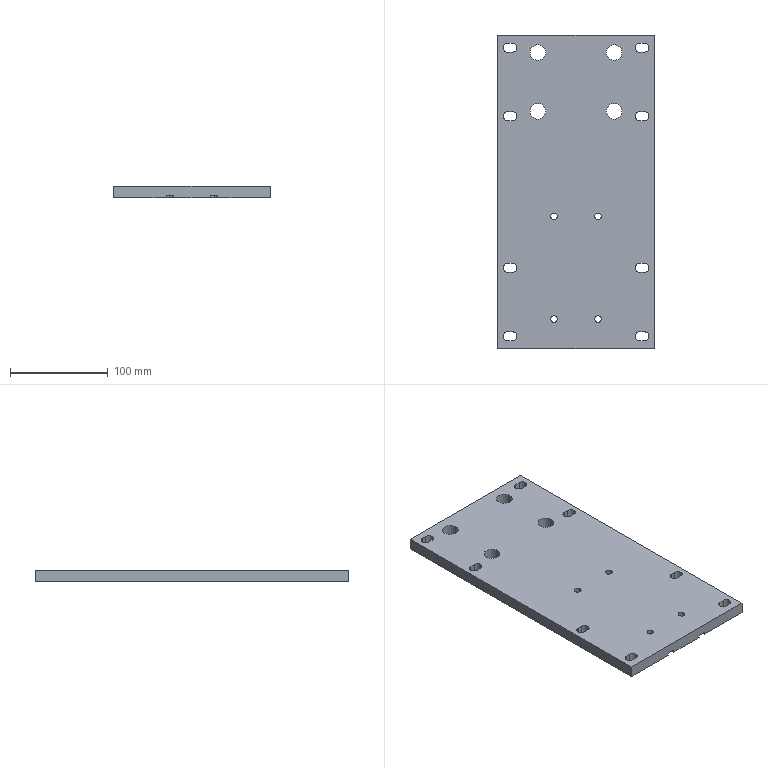Part | STEP file | X77-08301 | 1 solid | 136 faces | box 160 x 320 x 12 mm | volume 585549 mm3 | cylinder 76 | cone 32 | plane 28 | commonest cylinder face diameters 3.3 x32 9 x24 6.8 x8 16 x8 8 x4